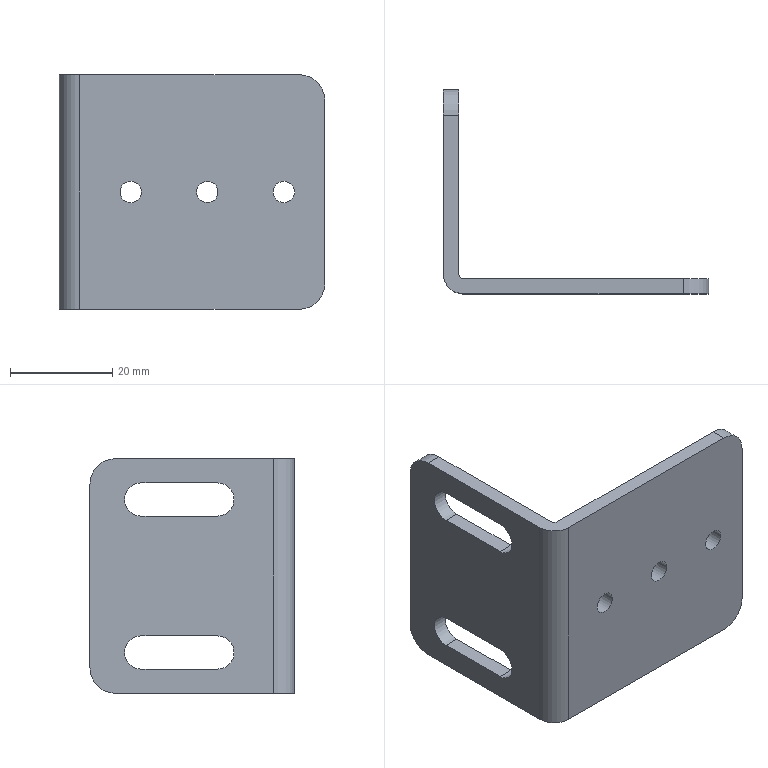Part | NX | features BREP 1 | 1 solid | 25 faces | box 52 x 40 x 46 mm | volume 11161 mm3 | cylinder 13 | plane 12 | commonest cylinder face diameters 6.5 x4 10 x4 4.2 x3 2 x1 8 x1
STEP:
#1=CARTESIAN_POINT('',(44.,0.,-2.1));
#2=VERTEX_POINT('',#1);
#3=CARTESIAN_POINT('',(44.,0.,0.));
#4=DIRECTION('',(0.,-1.,0.));
#5=DIRECTION('',(0.,0.,-1.));
#6=AXIS2_PLACEMENT_3D('',#3,#4,#5);
#7=CIRCLE('',#6,2.1);
#8=EDGE_CURVE('',#2,#2,#7,.T.);
#9=ORIENTED_EDGE('',*,*,#8,.T.);
#10=EDGE_LOOP('',(#9));
#11=FACE_BOUND('',#10,.T.);
#12=CARTESIAN_POINT('',(44.,3.,2.1));
#13=VERTEX_POINT('',#12);
#14=CARTESIAN_POINT('',(44.,3.,0.));
#15=DIRECTION('',(0.,1.,0.));
#16=DIRECTION('',(0.,0.,1.));
#17=AXIS2_PLACEMENT_3D('',#14,#15,#16);
#18=CIRCLE('',#17,2.1);
#19=EDGE_CURVE('',#13,#13,#18,.T.);
#20=ORIENTED_EDGE('',*,*,#19,.T.);
#21=EDGE_LOOP('',(#20));
#22=FACE_BOUND('',#21,.T.);
#23=CARTESIAN_POINT('',(44.,0.,0.));
#24=DIRECTION('',(0.,-1.,0.));
#25=DIRECTION('',(0.,0.,-1.));
#26=AXIS2_PLACEMENT_3D('',#23,#24,#25);
#27=CYLINDRICAL_SURFACE('',#26,2.1);
#28=ADVANCED_FACE('',(#11,#22),#27,.F.);
#29=CARTESIAN_POINT('',(14.,0.,-2.1));
#30=VERTEX_POINT('',#29);
#31=CARTESIAN_POINT('',(14.,0.,0.));
#32=DIRECTION('',(0.,-1.,0.));
#33=DIRECTION('',(0.,0.,-1.));
#34=AXIS2_PLACEMENT_3D('',#31,#32,#33);
#35=CIRCLE('',#34,2.1);
#36=EDGE_CURVE('',#30,#30,#35,.T.);
#37=ORIENTED_EDGE('',*,*,#36,.T.);
#38=EDGE_LOOP('',(#37));
#39=FACE_BOUND('',#38,.T.);
#40=CARTESIAN_POINT('',(14.,3.,2.1));
#41=VERTEX_POINT('',#40);
#42=CARTESIAN_POINT('',(14.,3.,0.));
#43=DIRECTION('',(0.,1.,0.));
#44=DIRECTION('',(0.,0.,1.));
#45=AXIS2_PLACEMENT_3D('',#42,#43,#44);
#46=CIRCLE('',#45,2.1);
#47=EDGE_CURVE('',#41,#41,#46,.T.);
#48=ORIENTED_EDGE('',*,*,#47,.T.);
#49=EDGE_LOOP('',(#48));
#50=FACE_BOUND('',#49,.T.);
#51=CARTESIAN_POINT('',(14.,0.,0.));
#52=DIRECTION('',(0.,-1.,0.));
#53=DIRECTION('',(0.,0.,-1.));
#54=AXIS2_PLACEMENT_3D('',#51,#52,#53);
#55=CYLINDRICAL_SURFACE('',#54,2.1);
#56=ADVANCED_FACE('',(#39,#50),#55,.F.);
#57=CARTESIAN_POINT('',(29.,0.,-2.1));
#58=VERTEX_POINT('',#57);
#59=CARTESIAN_POINT('',(29.,0.,0.));
#60=DIRECTION('',(0.,-1.,0.));
#61=DIRECTION('',(0.,0.,-1.));
#62=AXIS2_PLACEMENT_3D('',#59,#60,#61);
#63=CIRCLE('',#62,2.1);
#64=EDGE_CURVE('',#58,#58,#63,.T.);
#65=ORIENTED_EDGE('',*,*,#64,.T.);
#66=EDGE_LOOP('',(#65));
#67=FACE_BOUND('',#66,.T.);
#68=CARTESIAN_POINT('',(29.,3.,2.1));
#69=VERTEX_POINT('',#68);
#70=CARTESIAN_POINT('',(29.,3.,0.));
#71=DIRECTION('',(0.,1.,0.));
#72=DIRECTION('',(0.,0.,1.));
#73=AXIS2_PLACEMENT_3D('',#70,#71,#72);
#74=CIRCLE('',#73,2.1);
#75=EDGE_CURVE('',#69,#69,#74,.T.);
#76=ORIENTED_EDGE('',*,*,#75,.T.);
#77=EDGE_LOOP('',(#76));
#78=FACE_BOUND('',#77,.T.);
#79=CARTESIAN_POINT('',(29.,0.,0.));
#80=DIRECTION('',(0.,-1.,0.));
#81=DIRECTION('',(0.,0.,-1.));
#82=AXIS2_PLACEMENT_3D('',#79,#80,#81);
#83=CYLINDRICAL_SURFACE('',#82,2.1);
#84=ADVANCED_FACE('',(#67,#78),#83,.F.);
#85=CARTESIAN_POINT('',(3.,15.,-11.75));
#86=VERTEX_POINT('',#85);
#87=CARTESIAN_POINT('',(3.,15.,-18.25));
#88=VERTEX_POINT('',#87);
#89=CARTESIAN_POINT('',(3.,15.,-15.));
#90=DIRECTION('',(1.,0.,0.));
#91=DIRECTION('',(0.,1.,0.));
#92=AXIS2_PLACEMENT_3D('',#89,#90,#91);
#93=CIRCLE('',#92,3.25);
#94=EDGE_CURVE('',#86,#88,#93,.T.);
#95=ORIENTED_EDGE('',*,*,#94,.T.);
#96=CARTESIAN_POINT('',(0.,15.,-18.25));
#97=VERTEX_POINT('',#96);
#98=CARTESIAN_POINT('',(10.,15.,-18.25));
#99=DIRECTION('',(-1.,0.,0.));
#100=VECTOR('',#99,1000.);
#101=LINE('',#98,#100);
#102=EDGE_CURVE('',#88,#97,#101,.T.);
#103=ORIENTED_EDGE('',*,*,#102,.T.);
#104=CARTESIAN_POINT('',(0.,15.,-11.75));
#105=VERTEX_POINT('',#104);
#106=CARTESIAN_POINT('',(0.,15.,-15.));
#107=DIRECTION('',(-1.,0.,0.));
#108=DIRECTION('',(0.,1.,0.));
#109=AXIS2_PLACEMENT_3D('',#106,#107,#108);
#110=CIRCLE('',#109,3.25);
#111=EDGE_CURVE('',#97,#105,#110,.T.);
#112=ORIENTED_EDGE('',*,*,#111,.T.);
#113=CARTESIAN_POINT('',(10.,15.,-11.75));
#114=DIRECTION('',(-1.,0.,0.));
#115=VECTOR('',#114,1000.);
#116=LINE('',#113,#115);
#117=EDGE_CURVE('',#86,#105,#116,.T.);
#118=ORIENTED_EDGE('',*,*,#117,.F.);
#119=EDGE_LOOP('',(#95,#103,#112,#118));
#120=FACE_BOUND('',#119,.T.);
#121=CARTESIAN_POINT('',(10.,15.,-15.));
#122=DIRECTION('',(-1.,0.,0.));
#123=DIRECTION('',(0.,-1.,0.));
#124=AXIS2_PLACEMENT_3D('',#121,#122,#123);
#125=CYLINDRICAL_SURFACE('',#124,3.25);
#126=ADVANCED_FACE('',(#120),#125,.F.);
#127=CARTESIAN_POINT('',(3.,15.,18.25));
#128=VERTEX_POINT('',#127);
#129=CARTESIAN_POINT('',(3.,15.,11.75));
#130=VERTEX_POINT('',#129);
#131=CARTESIAN_POINT('',(3.,15.,15.));
#132=DIRECTION('',(1.,0.,0.));
#133=DIRECTION('',(0.,1.,0.));
#134=AXIS2_PLACEMENT_3D('',#131,#132,#133);
#135=CIRCLE('',#134,3.25);
#136=EDGE_CURVE('',#128,#130,#135,.T.);
#137=ORIENTED_EDGE('',*,*,#136,.T.);
#138=CARTESIAN_POINT('',(0.,15.,11.75));
#139=VERTEX_POINT('',#138);
#140=CARTESIAN_POINT('',(10.,15.,11.75));
#141=DIRECTION('',(-1.,0.,0.));
#142=VECTOR('',#141,1000.);
#143=LINE('',#140,#142);
#144=EDGE_CURVE('',#130,#139,#143,.T.);
#145=ORIENTED_EDGE('',*,*,#144,.T.);
#146=CARTESIAN_POINT('',(0.,15.,18.25));
#147=VERTEX_POINT('',#146);
#148=CARTESIAN_POINT('',(0.,15.,15.));
#149=DIRECTION('',(-1.,0.,0.));
#150=DIRECTION('',(0.,-1.,0.));
#151=AXIS2_PLACEMENT_3D('',#148,#149,#150);
#152=CIRCLE('',#151,3.25);
#153=EDGE_CURVE('',#139,#147,#152,.T.);
#154=ORIENTED_EDGE('',*,*,#153,.T.);
#155=CARTESIAN_POINT('',(10.,15.,18.25));
#156=DIRECTION('',(-1.,0.,0.));
#157=VECTOR('',#156,1000.);
#158=LINE('',#155,#157);
#159=EDGE_CURVE('',#128,#147,#158,.T.);
#160=ORIENTED_EDGE('',*,*,#159,.F.);
#161=EDGE_LOOP('',(#137,#145,#154,#160));
#162=FACE_BOUND('',#161,.T.);
#163=CARTESIAN_POINT('',(10.,15.,15.));
#164=DIRECTION('',(-1.,0.,0.));
#165=DIRECTION('',(0.,-1.,0.));
#166=AXIS2_PLACEMENT_3D('',#163,#164,#165);
#167=CYLINDRICAL_SURFACE('',#166,3.25);
#168=ADVANCED_FACE('',(#162),#167,.F.);
#169=CARTESIAN_POINT('',(3.,4.,23.));
#170=VERTEX_POINT('',#169);
#171=CARTESIAN_POINT('',(4.,3.,23.));
#172=VERTEX_POINT('',#171);
#173=CARTESIAN_POINT('',(4.,4.,23.));
#174=DIRECTION('',(0.,0.,1.));
#175=DIRECTION('',(1.,0.,0.));
#176=AXIS2_PLACEMENT_3D('',#173,#174,#175);
#177=CIRCLE('',#176,1.);
#178=EDGE_CURVE('',#170,#172,#177,.T.);
#179=ORIENTED_EDGE('',*,*,#178,.F.);
#180=CARTESIAN_POINT('',(3.,35.,23.));
#181=VERTEX_POINT('',#180);
#182=CARTESIAN_POINT('',(3.,40.,23.));
#183=DIRECTION('',(0.,-1.,0.));
#184=VECTOR('',#183,1000.);
#185=LINE('',#182,#184);
#186=EDGE_CURVE('',#181,#170,#185,.T.);
#187=ORIENTED_EDGE('',*,*,#186,.F.);
#188=CARTESIAN_POINT('',(0.,35.,23.));
#189=VERTEX_POINT('',#188);
#190=CARTESIAN_POINT('',(4.,35.,23.));
#191=DIRECTION('',(-1.,0.,0.));
#192=VECTOR('',#191,1000.);
#193=LINE('',#190,#192);
#194=EDGE_CURVE('',#181,#189,#193,.T.);
#195=ORIENTED_EDGE('',*,*,#194,.T.);
#196=CARTESIAN_POINT('',(0.,4.,23.));
#197=VERTEX_POINT('',#196);
#198=CARTESIAN_POINT('',(0.,40.,23.));
#199=DIRECTION('',(0.,-1.,0.));
#200=VECTOR('',#199,1000.);
#201=LINE('',#198,#200);
#202=EDGE_CURVE('',#189,#197,#201,.T.);
#203=ORIENTED_EDGE('',*,*,#202,.T.);
#204=CARTESIAN_POINT('',(4.,0.,23.));
#205=VERTEX_POINT('',#204);
#206=CARTESIAN_POINT('',(4.,4.,23.));
#207=DIRECTION('',(0.,0.,1.));
#208=DIRECTION('',(-1.,0.,0.));
#209=AXIS2_PLACEMENT_3D('',#206,#207,#208);
#210=CIRCLE('',#209,4.);
#211=EDGE_CURVE('',#197,#205,#210,.T.);
#212=ORIENTED_EDGE('',*,*,#211,.T.);
#213=CARTESIAN_POINT('',(47.,0.,23.));
#214=VERTEX_POINT('',#213);
#215=CARTESIAN_POINT('',(0.,0.,23.));
#216=DIRECTION('',(1.,0.,0.));
#217=VECTOR('',#216,1000.);
#218=LINE('',#215,#217);
#219=EDGE_CURVE('',#205,#214,#218,.T.);
#220=ORIENTED_EDGE('',*,*,#219,.T.);
#221=CARTESIAN_POINT('',(47.,3.,23.));
#222=VERTEX_POINT('',#221);
#223=CARTESIAN_POINT('',(47.,4.,23.));
#224=DIRECTION('',(0.,1.,0.));
#225=VECTOR('',#224,1000.);
#226=LINE('',#223,#225);
#227=EDGE_CURVE('',#214,#222,#226,.T.);
#228=ORIENTED_EDGE('',*,*,#227,.T.);
#229=CARTESIAN_POINT('',(0.,3.,23.));
#230=DIRECTION('',(1.,0.,0.));
#231=VECTOR('',#230,1000.);
#232=LINE('',#229,#231);
#233=EDGE_CURVE('',#172,#222,#232,.T.);
#234=ORIENTED_EDGE('',*,*,#233,.F.);
#235=EDGE_LOOP('',(#179,#187,#195,#203,#212,#220,#228,#234));
#236=FACE_BOUND('',#235,.T.);
#237=CARTESIAN_POINT('',(0.,4.,23.));
#238=DIRECTION('',(0.,0.,1.));
#239=DIRECTION('',(1.,0.,0.));
#240=AXIS2_PLACEMENT_3D('',#237,#238,#239);
#241=PLANE('',#240);
#242=ADVANCED_FACE('',(#236),#241,.T.);
#243=CARTESIAN_POINT('',(3.,4.,-23.));
#244=VERTEX_POINT('',#243);
#245=CARTESIAN_POINT('',(4.,3.,-23.));
#246=VERTEX_POINT('',#245);
#247=CARTESIAN_POINT('',(4.,4.,-23.));
#248=DIRECTION('',(0.,0.,1.));
#249=DIRECTION('',(1.,0.,0.));
#250=AXIS2_PLACEMENT_3D('',#247,#248,#249);
#251=CIRCLE('',#250,1.);
#252=EDGE_CURVE('',#244,#246,#251,.T.);
#253=ORIENTED_EDGE('',*,*,#252,.T.);
#254=CARTESIAN_POINT('',(47.,3.,-23.));
#255=VERTEX_POINT('',#254);
#256=CARTESIAN_POINT('',(0.,3.,-23.));
#257=DIRECTION('',(1.,0.,0.));
#258=VECTOR('',#257,1000.);
#259=LINE('',#256,#258);
#260=EDGE_CURVE('',#246,#255,#259,.T.);
#261=ORIENTED_EDGE('',*,*,#260,.T.);
#262=CARTESIAN_POINT('',(47.,0.,-23.));
#263=VERTEX_POINT('',#262);
#264=CARTESIAN_POINT('',(47.,4.,-23.));
#265=DIRECTION('',(0.,-1.,0.));
#266=VECTOR('',#265,1000.);
#267=LINE('',#264,#266);
#268=EDGE_CURVE('',#255,#263,#267,.T.);
#269=ORIENTED_EDGE('',*,*,#268,.T.);
#270=CARTESIAN_POINT('',(4.,0.,-23.));
#271=VERTEX_POINT('',#270);
#272=CARTESIAN_POINT('',(0.,0.,-23.));
#273=DIRECTION('',(1.,0.,0.));
#274=VECTOR('',#273,1000.);
#275=LINE('',#272,#274);
#276=EDGE_CURVE('',#271,#263,#275,.T.);
#277=ORIENTED_EDGE('',*,*,#276,.F.);
#278=CARTESIAN_POINT('',(0.,4.,-23.));
#279=VERTEX_POINT('',#278);
#280=CARTESIAN_POINT('',(4.,4.,-23.));
#281=DIRECTION('',(0.,0.,1.));
#282=DIRECTION('',(-1.,0.,0.));
#283=AXIS2_PLACEMENT_3D('',#280,#281,#282);
#284=CIRCLE('',#283,4.);
#285=EDGE_CURVE('',#279,#271,#284,.T.);
#286=ORIENTED_EDGE('',*,*,#285,.F.);
#287=CARTESIAN_POINT('',(0.,35.,-23.));
#288=VERTEX_POINT('',#287);
#289=CARTESIAN_POINT('',(0.,40.,-23.));
#290=DIRECTION('',(0.,-1.,0.));
#291=VECTOR('',#290,1000.);
#292=LINE('',#289,#291);
#293=EDGE_CURVE('',#288,#279,#292,.T.);
#294=ORIENTED_EDGE('',*,*,#293,.F.);
#295=CARTESIAN_POINT('',(3.,35.,-23.));
#296=VERTEX_POINT('',#295);
#297=CARTESIAN_POINT('',(3.,35.,-23.));
#298=DIRECTION('',(1.,0.,0.));
#299=VECTOR('',#298,1000.);
#300=LINE('',#297,#299);
#301=EDGE_CURVE('',#288,#296,#300,.T.);
#302=ORIENTED_EDGE('',*,*,#301,.T.);
#303=CARTESIAN_POINT('',(3.,40.,-23.));
#304=DIRECTION('',(0.,-1.,0.));
#305=VECTOR('',#304,1000.);
#306=LINE('',#303,#305);
#307=EDGE_CURVE('',#296,#244,#306,.T.);
#308=ORIENTED_EDGE('',*,*,#307,.T.);
#309=EDGE_LOOP('',(#253,#261,#269,#277,#286,#294,#302,#308));
#310=FACE_BOUND('',#309,.T.);
#311=CARTESIAN_POINT('',(4.,0.,-23.));
#312=DIRECTION('',(0.,0.,-1.));
#313=DIRECTION('',(-1.,0.,0.));
#314=AXIS2_PLACEMENT_3D('',#311,#312,#313);
#315=PLANE('',#314);
#316=ADVANCED_FACE('',(#310),#315,.T.);
#317=ORIENTED_EDGE('',*,*,#8,.F.);
#318=EDGE_LOOP('',(#317));
#319=FACE_BOUND('',#318,.T.);
#320=ORIENTED_EDGE('',*,*,#36,.F.);
#321=EDGE_LOOP('',(#320));
#322=FACE_BOUND('',#321,.T.);
#323=ORIENTED_EDGE('',*,*,#64,.F.);
#324=EDGE_LOOP('',(#323));
#325=FACE_BOUND('',#324,.T.);
#326=ORIENTED_EDGE('',*,*,#276,.T.);
#327=CARTESIAN_POINT('',(52.,0.,-18.));
#328=VERTEX_POINT('',#327);
#329=CARTESIAN_POINT('',(47.,0.,-18.));
#330=DIRECTION('',(0.,-1.,0.));
#331=DIRECTION('',(0.,0.,1.));
#332=AXIS2_PLACEMENT_3D('',#329,#330,#331);
#333=CIRCLE('',#332,5.);
#334=EDGE_CURVE('',#263,#328,#333,.T.);
#335=ORIENTED_EDGE('',*,*,#334,.T.);
#336=CARTESIAN_POINT('',(52.,0.,18.));
#337=VERTEX_POINT('',#336);
#338=CARTESIAN_POINT('',(52.,0.,23.));
#339=DIRECTION('',(0.,0.,-1.));
#340=VECTOR('',#339,1000.);
#341=LINE('',#338,#340);
#342=EDGE_CURVE('',#337,#328,#341,.T.);
#343=ORIENTED_EDGE('',*,*,#342,.F.);
#344=CARTESIAN_POINT('',(47.,0.,18.));
#345=DIRECTION('',(0.,-1.,0.));
#346=DIRECTION('',(0.,0.,1.));
#347=AXIS2_PLACEMENT_3D('',#344,#345,#346);
#348=CIRCLE('',#347,5.);
#349=EDGE_CURVE('',#337,#214,#348,.T.);
#350=ORIENTED_EDGE('',*,*,#349,.T.);
#351=ORIENTED_EDGE('',*,*,#219,.F.);
#352=CARTESIAN_POINT('',(4.,0.,23.));
#353=DIRECTION('',(0.,0.,-1.));
#354=VECTOR('',#353,1000.);
#355=LINE('',#352,#354);
#356=EDGE_CURVE('',#205,#271,#355,.T.);
#357=ORIENTED_EDGE('',*,*,#356,.T.);
#358=EDGE_LOOP('',(#326,#335,#343,#350,#351,#357));
#359=FACE_BOUND('',#358,.T.);
#360=CARTESIAN_POINT('',(0.,0.,23.));
#361=DIRECTION('',(0.,1.,0.));
#362=DIRECTION('',(0.,0.,1.));
#363=AXIS2_PLACEMENT_3D('',#360,#361,#362);
#364=PLANE('',#363);
#365=ADVANCED_FACE('',(#319,#322,#325,#359),#364,.F.);
#366=ORIENTED_EDGE('',*,*,#342,.T.);
#367=CARTESIAN_POINT('',(52.,3.,-18.));
#368=VERTEX_POINT('',#367);
#369=CARTESIAN_POINT('',(52.,3.,-18.));
#370=DIRECTION('',(0.,1.,0.));
#371=VECTOR('',#370,1000.);
#372=LINE('',#369,#371);
#373=EDGE_CURVE('',#328,#368,#372,.T.);
#374=ORIENTED_EDGE('',*,*,#373,.T.);
#375=CARTESIAN_POINT('',(52.,3.,18.));
#376=VERTEX_POINT('',#375);
#377=CARTESIAN_POINT('',(52.,3.,23.));
#378=DIRECTION('',(0.,0.,-1.));
#379=VECTOR('',#378,1000.);
#380=LINE('',#377,#379);
#381=EDGE_CURVE('',#376,#368,#380,.T.);
#382=ORIENTED_EDGE('',*,*,#381,.F.);
#383=CARTESIAN_POINT('',(52.,3.,18.));
#384=DIRECTION('',(0.,-1.,0.));
#385=VECTOR('',#384,1000.);
#386=LINE('',#383,#385);
#387=EDGE_CURVE('',#376,#337,#386,.T.);
#388=ORIENTED_EDGE('',*,*,#387,.T.);
#389=EDGE_LOOP('',(#366,#374,#382,#388));
#390=FACE_BOUND('',#389,.T.);
#391=CARTESIAN_POINT('',(52.,3.,23.));
#392=DIRECTION('',(1.,0.,0.));
#393=DIRECTION('',(0.,0.,-1.));
#394=AXIS2_PLACEMENT_3D('',#391,#392,#393);
#395=PLANE('',#394);
#396=ADVANCED_FACE('',(#390),#395,.T.);
#397=ORIENTED_EDGE('',*,*,#19,.F.);
#398=EDGE_LOOP('',(#397));
#399=FACE_BOUND('',#398,.T.);
#400=ORIENTED_EDGE('',*,*,#47,.F.);
#401=EDGE_LOOP('',(#400));
#402=FACE_BOUND('',#401,.T.);
#403=ORIENTED_EDGE('',*,*,#75,.F.);
#404=EDGE_LOOP('',(#403));
#405=FACE_BOUND('',#404,.T.);
#406=ORIENTED_EDGE('',*,*,#381,.T.);
#407=CARTESIAN_POINT('',(47.,3.,-18.));
#408=DIRECTION('',(0.,1.,0.));
#409=DIRECTION('',(0.,0.,1.));
#410=AXIS2_PLACEMENT_3D('',#407,#408,#409);
#411=CIRCLE('',#410,5.);
#412=EDGE_CURVE('',#368,#255,#411,.T.);
#413=ORIENTED_EDGE('',*,*,#412,.T.);
#414=ORIENTED_EDGE('',*,*,#260,.F.);
#415=CARTESIAN_POINT('',(4.,3.,23.));
#416=DIRECTION('',(0.,0.,-1.));
#417=VECTOR('',#416,1000.);
#418=LINE('',#415,#417);
#419=EDGE_CURVE('',#172,#246,#418,.T.);
#420=ORIENTED_EDGE('',*,*,#419,.F.);
#421=ORIENTED_EDGE('',*,*,#233,.T.);
#422=CARTESIAN_POINT('',(47.,3.,18.));
#423=DIRECTION('',(0.,1.,0.));
#424=DIRECTION('',(0.,0.,1.));
#425=AXIS2_PLACEMENT_3D('',#422,#423,#424);
#426=CIRCLE('',#425,5.);
#427=EDGE_CURVE('',#222,#376,#426,.T.);
#428=ORIENTED_EDGE('',*,*,#427,.T.);
#429=EDGE_LOOP('',(#406,#413,#414,#420,#421,#428));
#430=FACE_BOUND('',#429,.T.);
#431=CARTESIAN_POINT('',(0.,3.,23.));
#432=DIRECTION('',(0.,1.,0.));
#433=DIRECTION('',(0.,0.,1.));
#434=AXIS2_PLACEMENT_3D('',#431,#432,#433);
#435=PLANE('',#434);
#436=ADVANCED_FACE('',(#399,#402,#405,#430),#435,.T.);
#437=ORIENTED_EDGE('',*,*,#252,.F.);
#438=CARTESIAN_POINT('',(3.,4.,23.));
#439=DIRECTION('',(0.,0.,-1.));
#440=VECTOR('',#439,1000.);
#441=LINE('',#438,#440);
#442=EDGE_CURVE('',#170,#244,#441,.T.);
#443=ORIENTED_EDGE('',*,*,#442,.F.);
#444=ORIENTED_EDGE('',*,*,#178,.T.);
#445=ORIENTED_EDGE('',*,*,#419,.T.);
#446=EDGE_LOOP('',(#437,#443,#444,#445));
#447=FACE_BOUND('',#446,.T.);
#448=CARTESIAN_POINT('',(4.,4.,23.));
#449=DIRECTION('',(0.,0.,-1.));
#450=DIRECTION('',(-1.,0.,0.));
#451=AXIS2_PLACEMENT_3D('',#448,#449,#450);
#452=CYLINDRICAL_SURFACE('',#451,1.);
#453=ADVANCED_FACE('',(#447),#452,.F.);
#454=CARTESIAN_POINT('',(3.,30.,-18.25));
#455=VERTEX_POINT('',#454);
#456=CARTESIAN_POINT('',(3.,30.,-11.75));
#457=VERTEX_POINT('',#456);
#458=CARTESIAN_POINT('',(3.,30.,-15.));
#459=DIRECTION('',(1.,0.,0.));
#460=DIRECTION('',(0.,1.,0.));
#461=AXIS2_PLACEMENT_3D('',#458,#459,#460);
#462=CIRCLE('',#461,3.25);
#463=EDGE_CURVE('',#455,#457,#462,.T.);
#464=ORIENTED_EDGE('',*,*,#463,.F.);
#465=CARTESIAN_POINT('',(3.,40.,-18.25));
#466=DIRECTION('',(0.,1.,0.));
#467=VECTOR('',#466,1000.);
#468=LINE('',#465,#467);
#469=EDGE_CURVE('',#88,#455,#468,.T.);
#470=ORIENTED_EDGE('',*,*,#469,.F.);
#471=ORIENTED_EDGE('',*,*,#94,.F.);
#472=CARTESIAN_POINT('',(3.,40.,-11.75));
#473=DIRECTION('',(0.,-1.,0.));
#474=VECTOR('',#473,1000.);
#475=LINE('',#472,#474);
#476=EDGE_CURVE('',#457,#86,#475,.T.);
#477=ORIENTED_EDGE('',*,*,#476,.F.);
#478=EDGE_LOOP('',(#464,#470,#471,#477));
#479=FACE_BOUND('',#478,.T.);
#480=CARTESIAN_POINT('',(3.,30.,11.75));
#481=VERTEX_POINT('',#480);
#482=CARTESIAN_POINT('',(3.,30.,18.25));
#483=VERTEX_POINT('',#482);
#484=CARTESIAN_POINT('',(3.,30.,15.));
#485=DIRECTION('',(1.,0.,0.));
#486=DIRECTION('',(0.,1.,0.));
#487=AXIS2_PLACEMENT_3D('',#484,#485,#486);
#488=CIRCLE('',#487,3.25);
#489=EDGE_CURVE('',#481,#483,#488,.T.);
#490=ORIENTED_EDGE('',*,*,#489,.F.);
#491=CARTESIAN_POINT('',(3.,40.,11.75));
#492=DIRECTION('',(0.,1.,0.));
#493=VECTOR('',#492,1000.);
#494=LINE('',#491,#493);
#495=EDGE_CURVE('',#130,#481,#494,.T.);
#496=ORIENTED_EDGE('',*,*,#495,.F.);
#497=ORIENTED_EDGE('',*,*,#136,.F.);
#498=CARTESIAN_POINT('',(3.,40.,18.25));
#499=DIRECTION('',(0.,-1.,0.));
#500=VECTOR('',#499,1000.);
#501=LINE('',#498,#500);
#502=EDGE_CURVE('',#483,#128,#501,.T.);
#503=ORIENTED_EDGE('',*,*,#502,.F.);
#504=EDGE_LOOP('',(#490,#496,#497,#503));
#505=FACE_BOUND('',#504,.T.);
#506=ORIENTED_EDGE('',*,*,#307,.F.);
#507=CARTESIAN_POINT('',(3.,40.,-18.));
#508=VERTEX_POINT('',#507);
#509=CARTESIAN_POINT('',(3.,35.,-18.));
#510=DIRECTION('',(1.,0.,0.));
#511=DIRECTION('',(0.,1.,0.));
#512=AXIS2_PLACEMENT_3D('',#509,#510,#511);
#513=CIRCLE('',#512,5.);
#514=EDGE_CURVE('',#296,#508,#513,.T.);
#515=ORIENTED_EDGE('',*,*,#514,.T.);
#516=CARTESIAN_POINT('',(3.,40.,18.));
#517=VERTEX_POINT('',#516);
#518=CARTESIAN_POINT('',(3.,40.,23.));
#519=DIRECTION('',(0.,0.,-1.));
#520=VECTOR('',#519,1000.);
#521=LINE('',#518,#520);
#522=EDGE_CURVE('',#517,#508,#521,.T.);
#523=ORIENTED_EDGE('',*,*,#522,.F.);
#524=CARTESIAN_POINT('',(3.,35.,18.));
#525=DIRECTION('',(1.,0.,0.));
#526=DIRECTION('',(0.,1.,0.));
#527=AXIS2_PLACEMENT_3D('',#524,#525,#526);
#528=CIRCLE('',#527,5.);
#529=EDGE_CURVE('',#517,#181,#528,.T.);
#530=ORIENTED_EDGE('',*,*,#529,.T.);
#531=ORIENTED_EDGE('',*,*,#186,.T.);
#532=ORIENTED_EDGE('',*,*,#442,.T.);
#533=EDGE_LOOP('',(#506,#515,#523,#530,#531,#532));
#534=FACE_BOUND('',#533,.T.);
#535=CARTESIAN_POINT('',(3.,40.,23.));
#536=DIRECTION('',(1.,0.,0.));
#537=DIRECTION('',(0.,1.,0.));
#538=AXIS2_PLACEMENT_3D('',#535,#536,#537);
#539=PLANE('',#538);
#540=ADVANCED_FACE('',(#479,#505,#534),#539,.T.);
#541=ORIENTED_EDGE('',*,*,#522,.T.);
#542=CARTESIAN_POINT('',(0.,40.,-18.));
#543=VERTEX_POINT('',#542);
#544=CARTESIAN_POINT('',(0.,40.,-18.));
#545=DIRECTION('',(-1.,0.,0.));
#546=VECTOR('',#545,1000.);
#547=LINE('',#544,#546);
#548=EDGE_CURVE('',#508,#543,#547,.T.);
#549=ORIENTED_EDGE('',*,*,#548,.T.);
#550=CARTESIAN_POINT('',(0.,40.,18.));
#551=VERTEX_POINT('',#550);
#552=CARTESIAN_POINT('',(0.,40.,23.));
#553=DIRECTION('',(0.,0.,-1.));
#554=VECTOR('',#553,1000.);
#555=LINE('',#552,#554);
#556=EDGE_CURVE('',#551,#543,#555,.T.);
#557=ORIENTED_EDGE('',*,*,#556,.F.);
#558=CARTESIAN_POINT('',(0.,40.,18.));
#559=DIRECTION('',(1.,0.,0.));
#560=VECTOR('',#559,1000.);
#561=LINE('',#558,#560);
#562=EDGE_CURVE('',#551,#517,#561,.T.);
#563=ORIENTED_EDGE('',*,*,#562,.T.);
#564=EDGE_LOOP('',(#541,#549,#557,#563));
#565=FACE_BOUND('',#564,.T.);
#566=CARTESIAN_POINT('',(0.,40.,23.));
#567=DIRECTION('',(0.,1.,0.));
#568=DIRECTION('',(0.,0.,1.));
#569=AXIS2_PLACEMENT_3D('',#566,#567,#568);
#570=PLANE('',#569);
#571=ADVANCED_FACE('',(#565),#570,.T.);
#572=CARTESIAN_POINT('',(0.,30.,-18.25));
#573=VERTEX_POINT('',#572);
#574=CARTESIAN_POINT('',(0.,30.,-18.25));
#575=DIRECTION('',(0.,-1.,0.));
#576=VECTOR('',#575,1000.);
#577=LINE('',#574,#576);
#578=EDGE_CURVE('',#573,#97,#577,.T.);
#579=ORIENTED_EDGE('',*,*,#578,.F.);
#580=CARTESIAN_POINT('',(0.,30.,-11.75));
#581=VERTEX_POINT('',#580);
#582=CARTESIAN_POINT('',(0.,30.,-15.));
#583=DIRECTION('',(-1.,0.,0.));
#584=DIRECTION('',(0.,1.,0.));
#585=AXIS2_PLACEMENT_3D('',#582,#583,#584);
#586=CIRCLE('',#585,3.25);
#587=EDGE_CURVE('',#581,#573,#586,.T.);
#588=ORIENTED_EDGE('',*,*,#587,.F.);
#589=CARTESIAN_POINT('',(0.,30.,-11.75));
#590=DIRECTION('',(0.,1.,0.));
#591=VECTOR('',#590,1000.);
#592=LINE('',#589,#591);
#593=EDGE_CURVE('',#105,#581,#592,.T.);
#594=ORIENTED_EDGE('',*,*,#593,.F.);
#595=ORIENTED_EDGE('',*,*,#111,.F.);
#596=EDGE_LOOP('',(#579,#588,#594,#595));
#597=FACE_BOUND('',#596,.T.);
#598=CARTESIAN_POINT('',(0.,30.,11.75));
#599=VERTEX_POINT('',#598);
#600=CARTESIAN_POINT('',(0.,30.,11.75));
#601=DIRECTION('',(0.,-1.,0.));
#602=VECTOR('',#601,1000.);
#603=LINE('',#600,#602);
#604=EDGE_CURVE('',#599,#139,#603,.T.);
#605=ORIENTED_EDGE('',*,*,#604,.F.);
#606=CARTESIAN_POINT('',(0.,30.,18.25));
#607=VERTEX_POINT('',#606);
#608=CARTESIAN_POINT('',(0.,30.,15.));
#609=DIRECTION('',(-1.,0.,0.));
#610=DIRECTION('',(0.,-1.,0.));
#611=AXIS2_PLACEMENT_3D('',#608,#609,#610);
#612=CIRCLE('',#611,3.25);
#613=EDGE_CURVE('',#607,#599,#612,.T.);
#614=ORIENTED_EDGE('',*,*,#613,.F.);
#615=CARTESIAN_POINT('',(0.,30.,18.25));
#616=DIRECTION('',(0.,1.,0.));
#617=VECTOR('',#616,1000.);
#618=LINE('',#615,#617);
#619=EDGE_CURVE('',#147,#607,#618,.T.);
#620=ORIENTED_EDGE('',*,*,#619,.F.);
#621=ORIENTED_EDGE('',*,*,#153,.F.);
#622=EDGE_LOOP('',(#605,#614,#620,#621));
#623=FACE_BOUND('',#622,.T.);
#624=ORIENTED_EDGE('',*,*,#556,.T.);
#625=CARTESIAN_POINT('',(0.,35.,-18.));
#626=DIRECTION('',(-1.,0.,0.));
#627=DIRECTION('',(0.,1.,0.));
#628=AXIS2_PLACEMENT_3D('',#625,#626,#627);
#629=CIRCLE('',#628,5.);
#630=EDGE_CURVE('',#543,#288,#629,.T.);
#631=ORIENTED_EDGE('',*,*,#630,.T.);
#632=ORIENTED_EDGE('',*,*,#293,.T.);
#633=CARTESIAN_POINT('',(0.,4.,23.));
#634=DIRECTION('',(0.,0.,-1.));
#635=VECTOR('',#634,1000.);
#636=LINE('',#633,#635);
#637=EDGE_CURVE('',#197,#279,#636,.T.);
#638=ORIENTED_EDGE('',*,*,#637,.F.);
#639=ORIENTED_EDGE('',*,*,#202,.F.);
#640=CARTESIAN_POINT('',(0.,35.,18.));
#641=DIRECTION('',(-1.,0.,0.));
#642=DIRECTION('',(0.,1.,0.));
#643=AXIS2_PLACEMENT_3D('',#640,#641,#642);
#644=CIRCLE('',#643,5.);
#645=EDGE_CURVE('',#189,#551,#644,.T.);
#646=ORIENTED_EDGE('',*,*,#645,.T.);
#647=EDGE_LOOP('',(#624,#631,#632,#638,#639,#646));
#648=FACE_BOUND('',#647,.T.);
#649=CARTESIAN_POINT('',(0.,40.,23.));
#650=DIRECTION('',(1.,0.,0.));
#651=DIRECTION('',(0.,1.,0.));
#652=AXIS2_PLACEMENT_3D('',#649,#650,#651);
#653=PLANE('',#652);
#654=ADVANCED_FACE('',(#597,#623,#648),#653,.F.);
#655=ORIENTED_EDGE('',*,*,#285,.T.);
#656=ORIENTED_EDGE('',*,*,#356,.F.);
#657=ORIENTED_EDGE('',*,*,#211,.F.);
#658=ORIENTED_EDGE('',*,*,#637,.T.);
#659=EDGE_LOOP('',(#655,#656,#657,#658));
#660=FACE_BOUND('',#659,.T.);
#661=CARTESIAN_POINT('',(4.,4.,23.));
#662=DIRECTION('',(0.,0.,-1.));
#663=DIRECTION('',(-1.,0.,0.));
#664=AXIS2_PLACEMENT_3D('',#661,#662,#663);
#665=CYLINDRICAL_SURFACE('',#664,4.);
#666=ADVANCED_FACE('',(#660),#665,.T.);
#667=ORIENTED_EDGE('',*,*,#630,.F.);
#668=ORIENTED_EDGE('',*,*,#548,.F.);
#669=ORIENTED_EDGE('',*,*,#514,.F.);
#670=ORIENTED_EDGE('',*,*,#301,.F.);
#671=EDGE_LOOP('',(#667,#668,#669,#670));
#672=FACE_BOUND('',#671,.T.);
#673=CARTESIAN_POINT('',(4.,35.,-18.));
#674=DIRECTION('',(-1.,0.,0.));
#675=DIRECTION('',(0.,0.,1.));
#676=AXIS2_PLACEMENT_3D('',#673,#674,#675);
#677=CYLINDRICAL_SURFACE('',#676,5.);
#678=ADVANCED_FACE('',(#672),#677,.T.);
#679=ORIENTED_EDGE('',*,*,#645,.F.);
#680=ORIENTED_EDGE('',*,*,#194,.F.);
#681=ORIENTED_EDGE('',*,*,#529,.F.);
#682=ORIENTED_EDGE('',*,*,#562,.F.);
#683=EDGE_LOOP('',(#679,#680,#681,#682));
#684=FACE_BOUND('',#683,.T.);
#685=CARTESIAN_POINT('',(0.,35.,18.));
#686=DIRECTION('',(1.,0.,0.));
#687=DIRECTION('',(0.,0.,-1.));
#688=AXIS2_PLACEMENT_3D('',#685,#686,#687);
#689=CYLINDRICAL_SURFACE('',#688,5.);
#690=ADVANCED_FACE('',(#684),#689,.T.);
#691=ORIENTED_EDGE('',*,*,#412,.F.);
#692=ORIENTED_EDGE('',*,*,#373,.F.);
#693=ORIENTED_EDGE('',*,*,#334,.F.);
#694=ORIENTED_EDGE('',*,*,#268,.F.);
#695=EDGE_LOOP('',(#691,#692,#693,#694));
#696=FACE_BOUND('',#695,.T.);
#697=CARTESIAN_POINT('',(47.,4.,-18.));
#698=DIRECTION('',(0.,-1.,0.));
#699=DIRECTION('',(0.,0.,-1.));
#700=AXIS2_PLACEMENT_3D('',#697,#698,#699);
#701=CYLINDRICAL_SURFACE('',#700,5.);
#702=ADVANCED_FACE('',(#696),#701,.T.);
#703=ORIENTED_EDGE('',*,*,#427,.F.);
#704=ORIENTED_EDGE('',*,*,#227,.F.);
#705=ORIENTED_EDGE('',*,*,#349,.F.);
#706=ORIENTED_EDGE('',*,*,#387,.F.);
#707=EDGE_LOOP('',(#703,#704,#705,#706));
#708=FACE_BOUND('',#707,.T.);
#709=CARTESIAN_POINT('',(47.,3.,18.));
#710=DIRECTION('',(0.,-1.,0.));
#711=DIRECTION('',(0.,0.,-1.));
#712=AXIS2_PLACEMENT_3D('',#709,#710,#711);
#713=CYLINDRICAL_SURFACE('',#712,5.);
#714=ADVANCED_FACE('',(#708),#713,.T.);
#715=ORIENTED_EDGE('',*,*,#489,.T.);
#716=CARTESIAN_POINT('',(10.,30.,18.25));
#717=DIRECTION('',(-1.,0.,0.));
#718=VECTOR('',#717,1000.);
#719=LINE('',#716,#718);
#720=EDGE_CURVE('',#483,#607,#719,.T.);
#721=ORIENTED_EDGE('',*,*,#720,.T.);
#722=ORIENTED_EDGE('',*,*,#613,.T.);
#723=CARTESIAN_POINT('',(10.,30.,11.75));
#724=DIRECTION('',(-1.,0.,0.));
#725=VECTOR('',#724,1000.);
#726=LINE('',#723,#725);
#727=EDGE_CURVE('',#481,#599,#726,.T.);
#728=ORIENTED_EDGE('',*,*,#727,.F.);
#729=EDGE_LOOP('',(#715,#721,#722,#728));
#730=FACE_BOUND('',#729,.T.);
#731=CARTESIAN_POINT('',(10.,30.,15.));
#732=DIRECTION('',(-1.,0.,0.));
#733=DIRECTION('',(0.,-1.,0.));
#734=AXIS2_PLACEMENT_3D('',#731,#732,#733);
#735=CYLINDRICAL_SURFACE('',#734,3.25);
#736=ADVANCED_FACE('',(#730),#735,.F.);
#737=ORIENTED_EDGE('',*,*,#502,.T.);
#738=ORIENTED_EDGE('',*,*,#159,.T.);
#739=ORIENTED_EDGE('',*,*,#619,.T.);
#740=ORIENTED_EDGE('',*,*,#720,.F.);
#741=EDGE_LOOP('',(#737,#738,#739,#740));
#742=FACE_BOUND('',#741,.T.);
#743=CARTESIAN_POINT('',(10.,30.,18.25));
#744=DIRECTION('',(0.,0.,1.));
#745=DIRECTION('',(0.,-1.,0.));
#746=AXIS2_PLACEMENT_3D('',#743,#744,#745);
#747=PLANE('',#746);
#748=ADVANCED_FACE('',(#742),#747,.F.);
#749=ORIENTED_EDGE('',*,*,#495,.T.);
#750=ORIENTED_EDGE('',*,*,#727,.T.);
#751=ORIENTED_EDGE('',*,*,#604,.T.);
#752=ORIENTED_EDGE('',*,*,#144,.F.);
#753=EDGE_LOOP('',(#749,#750,#751,#752));
#754=FACE_BOUND('',#753,.T.);
#755=CARTESIAN_POINT('',(10.,30.,11.75));
#756=DIRECTION('',(0.,0.,-1.));
#757=DIRECTION('',(-1.,0.,0.));
#758=AXIS2_PLACEMENT_3D('',#755,#756,#757);
#759=PLANE('',#758);
#760=ADVANCED_FACE('',(#754),#759,.F.);
#761=ORIENTED_EDGE('',*,*,#463,.T.);
#762=CARTESIAN_POINT('',(10.,30.,-11.75));
#763=DIRECTION('',(-1.,0.,0.));
#764=VECTOR('',#763,1000.);
#765=LINE('',#762,#764);
#766=EDGE_CURVE('',#457,#581,#765,.T.);
#767=ORIENTED_EDGE('',*,*,#766,.T.);
#768=ORIENTED_EDGE('',*,*,#587,.T.);
#769=CARTESIAN_POINT('',(10.,30.,-18.25));
#770=DIRECTION('',(-1.,0.,0.));
#771=VECTOR('',#770,1000.);
#772=LINE('',#769,#771);
#773=EDGE_CURVE('',#455,#573,#772,.T.);
#774=ORIENTED_EDGE('',*,*,#773,.F.);
#775=EDGE_LOOP('',(#761,#767,#768,#774));
#776=FACE_BOUND('',#775,.T.);
#777=CARTESIAN_POINT('',(10.,30.,-15.));
#778=DIRECTION('',(-1.,0.,0.));
#779=DIRECTION('',(0.,-1.,0.));
#780=AXIS2_PLACEMENT_3D('',#777,#778,#779);
#781=CYLINDRICAL_SURFACE('',#780,3.25);
#782=ADVANCED_FACE('',(#776),#781,.F.);
#783=ORIENTED_EDGE('',*,*,#476,.T.);
#784=ORIENTED_EDGE('',*,*,#117,.T.);
#785=ORIENTED_EDGE('',*,*,#593,.T.);
#786=ORIENTED_EDGE('',*,*,#766,.F.);
#787=EDGE_LOOP('',(#783,#784,#785,#786));
#788=FACE_BOUND('',#787,.T.);
#789=CARTESIAN_POINT('',(10.,30.,-11.75));
#790=DIRECTION('',(0.,0.,1.));
#791=DIRECTION('',(1.,0.,0.));
#792=AXIS2_PLACEMENT_3D('',#789,#790,#791);
#793=PLANE('',#792);
#794=ADVANCED_FACE('',(#788),#793,.F.);
#795=ORIENTED_EDGE('',*,*,#469,.T.);
#796=ORIENTED_EDGE('',*,*,#773,.T.);
#797=ORIENTED_EDGE('',*,*,#578,.T.);
#798=ORIENTED_EDGE('',*,*,#102,.F.);
#799=EDGE_LOOP('',(#795,#796,#797,#798));
#800=FACE_BOUND('',#799,.T.);
#801=CARTESIAN_POINT('',(10.,30.,-18.25));
#802=DIRECTION('',(0.,0.,-1.));
#803=DIRECTION('',(0.,1.,0.));
#804=AXIS2_PLACEMENT_3D('',#801,#802,#803);
#805=PLANE('',#804);
#806=ADVANCED_FACE('',(#800),#805,.F.);
#807=CLOSED_SHELL('',(#28,#56,#84,#126,#168,#242,#316,#365,#396,#436,#453,#540,#571,#654,#666,#678,#690,#702,#714,#736,#748,#760,#782,#794,#806));
#808=MANIFOLD_SOLID_BREP('',#807);
#809=(LENGTH_UNIT()NAMED_UNIT(*)SI_UNIT(.MILLI.,.METRE.));
#810=UNCERTAINTY_MEASURE_WITH_UNIT(LENGTH_MEASURE(0.00001),#809,'','');
#811=(NAMED_UNIT(*)PLANE_ANGLE_UNIT()SI_UNIT($,.RADIAN.));
#812=(NAMED_UNIT(*)SI_UNIT($,.STERADIAN.)SOLID_ANGLE_UNIT());
#813=(GEOMETRIC_REPRESENTATION_CONTEXT(3)GLOBAL_UNCERTAINTY_ASSIGNED_CONTEXT((#810))GLOBAL_UNIT_ASSIGNED_CONTEXT((#809,#811,#812))REPRESENTATION_CONTEXT('',''));
#814=ADVANCED_BREP_SHAPE_REPRESENTATION('',(#808),#813);